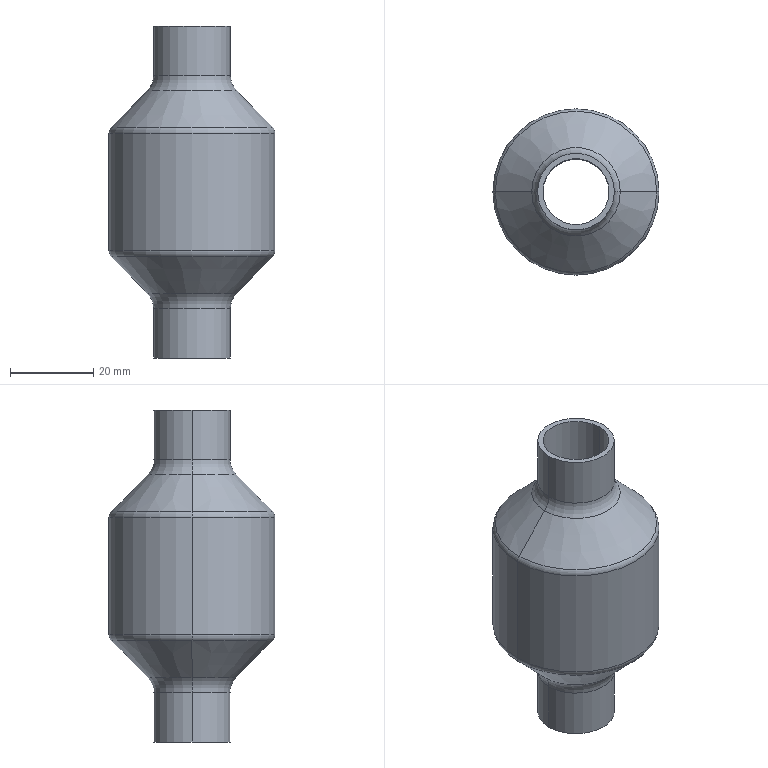Part | STEP file | filter | 1 solid | 30 faces | box 40 x 40 x 80 mm | volume 10214 mm3 | cylinder 12 | torus 8 | cone 8 | plane 2 | commonest cylinder face diameters 15.9 x4 18.5 x4 37.4 x2 40 x2